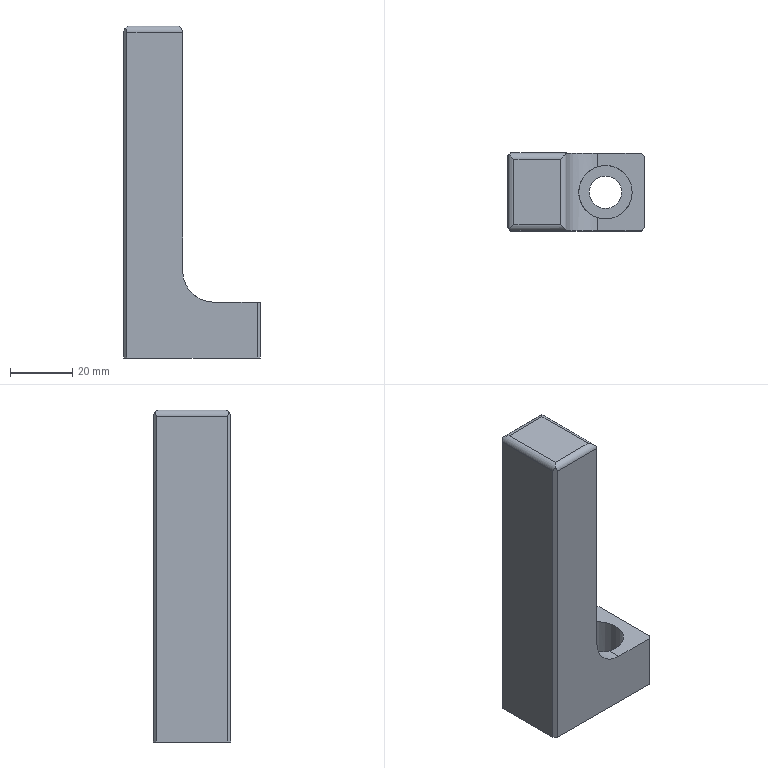Part | STEP file | 1_id670_x_t | 1 solid | 20 faces | box 44 x 25 x 107.009 mm | volume 59060 mm3 | plane 13 | cylinder 7 | commonest cylinder face diameters 4 x4 10.5 x1 17.25 x1 20 x1